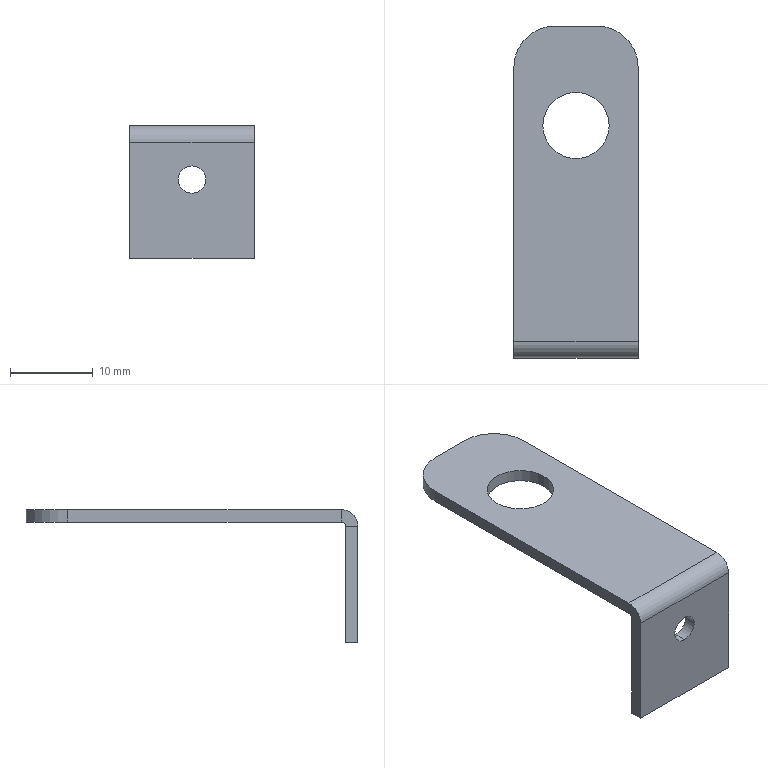Part | SolidWorks | features EdgeFlange 2, Fillet 2, FlatPattern 1, HoleWzd 1, ICE 1, SMBaseFlange 1, SheetMetal 1 | 1 solid | 20 faces | box 15 x 40 x 16 mm | volume 1110 mm3 | plane 12 | cylinder 8 | commonest cylinder face diameters 3.3 x2 8 x2 10 x2 1 x1 4 x1
STEP:
#1=CARTESIAN_POINT('',(4.,8.,0.));
#2=VERTEX_POINT('',#1);
#3=CARTESIAN_POINT('',(-4.,8.,0.));
#4=VERTEX_POINT('',#3);
#5=CARTESIAN_POINT('',(0.,8.,0.));
#6=DIRECTION('',(0.,0.,-1.));
#7=DIRECTION('',(-1.,0.,0.));
#8=AXIS2_PLACEMENT_3D('',#5,#6,#7);
#9=CIRCLE('',#8,4.);
#10=EDGE_CURVE('',#2,#4,#9,.T.);
#11=ORIENTED_EDGE('',*,*,#10,.F.);
#12=CARTESIAN_POINT('',(4.,8.,-1.5));
#13=VERTEX_POINT('',#12);
#14=CARTESIAN_POINT('',(4.,8.,0.));
#15=DIRECTION('',(0.,0.,-1.));
#16=VECTOR('',#15,1000.);
#17=LINE('',#14,#16);
#18=EDGE_CURVE('',#2,#13,#17,.T.);
#19=ORIENTED_EDGE('',*,*,#18,.T.);
#20=CARTESIAN_POINT('',(-4.,8.,-1.5));
#21=VERTEX_POINT('',#20);
#22=CARTESIAN_POINT('',(0.,8.,-1.5));
#23=DIRECTION('',(0.,0.,-1.));
#24=DIRECTION('',(-1.,0.,0.));
#25=AXIS2_PLACEMENT_3D('',#22,#23,#24);
#26=CIRCLE('',#25,4.);
#27=EDGE_CURVE('',#13,#21,#26,.T.);
#28=ORIENTED_EDGE('',*,*,#27,.T.);
#29=CARTESIAN_POINT('',(-4.,8.,0.));
#30=DIRECTION('',(0.,0.,-1.));
#31=VECTOR('',#30,1000.);
#32=LINE('',#29,#31);
#33=EDGE_CURVE('',#4,#21,#32,.T.);
#34=ORIENTED_EDGE('',*,*,#33,.F.);
#35=EDGE_LOOP('',(#11,#19,#28,#34));
#36=FACE_OUTER_BOUND('',#35,.T.);
#37=CARTESIAN_POINT('',(0.,8.,0.));
#38=DIRECTION('',(0.,0.,-1.));
#39=DIRECTION('',(-1.,0.,0.));
#40=AXIS2_PLACEMENT_3D('',#37,#38,#39);
#41=CYLINDRICAL_SURFACE('',#40,4.);
#42=ADVANCED_FACE('',(#36),#41,.F.);
#43=CARTESIAN_POINT('',(0.,-18.5,-4.85));
#44=VERTEX_POINT('',#43);
#45=CARTESIAN_POINT('',(0.,-18.5,-8.15));
#46=VERTEX_POINT('',#45);
#47=CARTESIAN_POINT('',(0.,-18.5,-6.5));
#48=DIRECTION('',(0.,-1.,0.));
#49=DIRECTION('',(0.,0.,-1.));
#50=AXIS2_PLACEMENT_3D('',#47,#48,#49);
#51=CIRCLE('',#50,1.65);
#52=EDGE_CURVE('',#44,#46,#51,.T.);
#53=ORIENTED_EDGE('',*,*,#52,.F.);
#54=CARTESIAN_POINT('',(0.,-20.,-4.85));
#55=VERTEX_POINT('',#54);
#56=CARTESIAN_POINT('',(0.,-20.,-4.85));
#57=DIRECTION('',(0.,-1.,0.));
#58=VECTOR('',#57,1000.);
#59=LINE('',#56,#58);
#60=EDGE_CURVE('',#44,#55,#59,.T.);
#61=ORIENTED_EDGE('',*,*,#60,.T.);
#62=CARTESIAN_POINT('',(0.,-20.,-8.15));
#63=VERTEX_POINT('',#62);
#64=CARTESIAN_POINT('',(0.,-20.,-6.5));
#65=DIRECTION('',(0.,-1.,0.));
#66=DIRECTION('',(0.,0.,-1.));
#67=AXIS2_PLACEMENT_3D('',#64,#65,#66);
#68=CIRCLE('',#67,1.65);
#69=EDGE_CURVE('',#55,#63,#68,.T.);
#70=ORIENTED_EDGE('',*,*,#69,.T.);
#71=CARTESIAN_POINT('',(0.,-20.,-8.15));
#72=DIRECTION('',(0.,-1.,0.));
#73=VECTOR('',#72,1000.);
#74=LINE('',#71,#73);
#75=EDGE_CURVE('',#46,#63,#74,.T.);
#76=ORIENTED_EDGE('',*,*,#75,.F.);
#77=EDGE_LOOP('',(#53,#61,#70,#76));
#78=FACE_OUTER_BOUND('',#77,.T.);
#79=CARTESIAN_POINT('',(0.,-20.,-6.5));
#80=DIRECTION('',(0.,-1.,0.));
#81=DIRECTION('',(0.,0.,-1.));
#82=AXIS2_PLACEMENT_3D('',#79,#80,#81);
#83=CYLINDRICAL_SURFACE('',#82,1.65);
#84=ADVANCED_FACE('',(#78),#83,.F.);
#85=CARTESIAN_POINT('',(-7.5,15.,-1.5));
#86=VERTEX_POINT('',#85);
#87=CARTESIAN_POINT('',(-7.5,-18.,-1.5));
#88=VERTEX_POINT('',#87);
#89=CARTESIAN_POINT('',(-7.5,-20.,-1.5));
#90=DIRECTION('',(0.,-1.,0.));
#91=VECTOR('',#90,1000.);
#92=LINE('',#89,#91);
#93=EDGE_CURVE('',#86,#88,#92,.T.);
#94=ORIENTED_EDGE('',*,*,#93,.T.);
#95=CARTESIAN_POINT('',(-7.5,-18.,0.));
#96=VERTEX_POINT('',#95);
#97=CARTESIAN_POINT('',(-7.5,-18.,-1.5));
#98=DIRECTION('',(0.,0.,1.));
#99=VECTOR('',#98,1000.);
#100=LINE('',#97,#99);
#101=EDGE_CURVE('',#88,#96,#100,.T.);
#102=ORIENTED_EDGE('',*,*,#101,.T.);
#103=CARTESIAN_POINT('',(-7.5,15.,0.));
#104=VERTEX_POINT('',#103);
#105=CARTESIAN_POINT('',(-7.5,-20.,0.));
#106=DIRECTION('',(0.,-1.,0.));
#107=VECTOR('',#106,1000.);
#108=LINE('',#105,#107);
#109=EDGE_CURVE('',#104,#96,#108,.T.);
#110=ORIENTED_EDGE('',*,*,#109,.F.);
#111=CARTESIAN_POINT('',(-7.5,15.,-1.5));
#112=DIRECTION('',(0.,0.,-1.));
#113=VECTOR('',#112,1000.);
#114=LINE('',#111,#113);
#115=EDGE_CURVE('',#104,#86,#114,.T.);
#116=ORIENTED_EDGE('',*,*,#115,.T.);
#117=EDGE_LOOP('',(#94,#102,#110,#116));
#118=FACE_OUTER_BOUND('',#117,.T.);
#119=CARTESIAN_POINT('',(-7.5,-20.,-1.5));
#120=DIRECTION('',(-1.,0.,0.));
#121=DIRECTION('',(0.,0.,1.));
#122=AXIS2_PLACEMENT_3D('',#119,#120,#121);
#123=PLANE('',#122);
#124=ADVANCED_FACE('',(#118),#123,.T.);
#125=CARTESIAN_POINT('',(0.,8.,-1.5));
#126=DIRECTION('',(0.,0.,-1.));
#127=DIRECTION('',(-1.,0.,0.));
#128=AXIS2_PLACEMENT_3D('',#125,#126,#127);
#129=CIRCLE('',#128,4.);
#130=EDGE_CURVE('',#21,#13,#129,.T.);
#131=ORIENTED_EDGE('',*,*,#130,.F.);
#132=ORIENTED_EDGE('',*,*,#27,.F.);
#133=EDGE_LOOP('',(#131,#132));
#134=FACE_BOUND('',#133,.T.);
#135=CARTESIAN_POINT('',(7.5,-18.,-1.5));
#136=VERTEX_POINT('',#135);
#137=CARTESIAN_POINT('',(-7.5,-18.,-1.5));
#138=DIRECTION('',(1.,0.,0.));
#139=VECTOR('',#138,1000.);
#140=LINE('',#137,#139);
#141=EDGE_CURVE('',#88,#136,#140,.T.);
#142=ORIENTED_EDGE('',*,*,#141,.F.);
#143=ORIENTED_EDGE('',*,*,#93,.F.);
#144=CARTESIAN_POINT('',(-2.5,20.,-1.5));
#145=VERTEX_POINT('',#144);
#146=CARTESIAN_POINT('',(-2.5,15.,-1.5));
#147=DIRECTION('',(0.,0.,-1.));
#148=DIRECTION('',(1.,0.,0.));
#149=AXIS2_PLACEMENT_3D('',#146,#147,#148);
#150=CIRCLE('',#149,5.);
#151=EDGE_CURVE('',#86,#145,#150,.T.);
#152=ORIENTED_EDGE('',*,*,#151,.T.);
#153=CARTESIAN_POINT('',(2.5,20.,-1.5));
#154=VERTEX_POINT('',#153);
#155=CARTESIAN_POINT('',(7.5,20.,-1.5));
#156=DIRECTION('',(-1.,0.,0.));
#157=VECTOR('',#156,1000.);
#158=LINE('',#155,#157);
#159=EDGE_CURVE('',#154,#145,#158,.T.);
#160=ORIENTED_EDGE('',*,*,#159,.F.);
#161=CARTESIAN_POINT('',(7.5,15.,-1.5));
#162=VERTEX_POINT('',#161);
#163=CARTESIAN_POINT('',(2.5,15.,-1.5));
#164=DIRECTION('',(0.,0.,-1.));
#165=DIRECTION('',(1.,0.,0.));
#166=AXIS2_PLACEMENT_3D('',#163,#164,#165);
#167=CIRCLE('',#166,5.);
#168=EDGE_CURVE('',#154,#162,#167,.T.);
#169=ORIENTED_EDGE('',*,*,#168,.T.);
#170=CARTESIAN_POINT('',(7.5,-20.,-1.5));
#171=DIRECTION('',(0.,1.,0.));
#172=VECTOR('',#171,1000.);
#173=LINE('',#170,#172);
#174=EDGE_CURVE('',#136,#162,#173,.T.);
#175=ORIENTED_EDGE('',*,*,#174,.F.);
#176=EDGE_LOOP('',(#142,#143,#152,#160,#169,#175));
#177=FACE_OUTER_BOUND('',#176,.T.);
#178=CARTESIAN_POINT('',(0.,0.,-1.5));
#179=DIRECTION('',(0.,0.,1.));
#180=DIRECTION('',(1.,0.,0.));
#181=AXIS2_PLACEMENT_3D('',#178,#179,#180);
#182=PLANE('',#181);
#183=ADVANCED_FACE('',(#134,#177),#182,.F.);
#184=CARTESIAN_POINT('',(0.,8.,0.));
#185=DIRECTION('',(0.,0.,-1.));
#186=DIRECTION('',(-1.,0.,0.));
#187=AXIS2_PLACEMENT_3D('',#184,#185,#186);
#188=CIRCLE('',#187,4.);
#189=EDGE_CURVE('',#4,#2,#188,.T.);
#190=ORIENTED_EDGE('',*,*,#189,.T.);
#191=ORIENTED_EDGE('',*,*,#10,.T.);
#192=EDGE_LOOP('',(#190,#191));
#193=FACE_BOUND('',#192,.T.);
#194=ORIENTED_EDGE('',*,*,#109,.T.);
#195=CARTESIAN_POINT('',(7.5,-18.,0.));
#196=VERTEX_POINT('',#195);
#197=CARTESIAN_POINT('',(-7.5,-18.,0.));
#198=DIRECTION('',(1.,0.,0.));
#199=VECTOR('',#198,1000.);
#200=LINE('',#197,#199);
#201=EDGE_CURVE('',#96,#196,#200,.T.);
#202=ORIENTED_EDGE('',*,*,#201,.T.);
#203=CARTESIAN_POINT('',(7.5,15.,0.));
#204=VERTEX_POINT('',#203);
#205=CARTESIAN_POINT('',(7.5,-20.,0.));
#206=DIRECTION('',(0.,1.,0.));
#207=VECTOR('',#206,1000.);
#208=LINE('',#205,#207);
#209=EDGE_CURVE('',#196,#204,#208,.T.);
#210=ORIENTED_EDGE('',*,*,#209,.T.);
#211=CARTESIAN_POINT('',(2.5,20.,0.));
#212=VERTEX_POINT('',#211);
#213=CARTESIAN_POINT('',(2.5,15.,0.));
#214=DIRECTION('',(0.,0.,1.));
#215=DIRECTION('',(1.,0.,0.));
#216=AXIS2_PLACEMENT_3D('',#213,#214,#215);
#217=CIRCLE('',#216,5.);
#218=EDGE_CURVE('',#204,#212,#217,.T.);
#219=ORIENTED_EDGE('',*,*,#218,.T.);
#220=CARTESIAN_POINT('',(-2.5,20.,0.));
#221=VERTEX_POINT('',#220);
#222=CARTESIAN_POINT('',(7.5,20.,0.));
#223=DIRECTION('',(-1.,0.,0.));
#224=VECTOR('',#223,1000.);
#225=LINE('',#222,#224);
#226=EDGE_CURVE('',#212,#221,#225,.T.);
#227=ORIENTED_EDGE('',*,*,#226,.T.);
#228=CARTESIAN_POINT('',(-2.5,15.,0.));
#229=DIRECTION('',(0.,0.,1.));
#230=DIRECTION('',(1.,0.,0.));
#231=AXIS2_PLACEMENT_3D('',#228,#229,#230);
#232=CIRCLE('',#231,5.);
#233=EDGE_CURVE('',#221,#104,#232,.T.);
#234=ORIENTED_EDGE('',*,*,#233,.T.);
#235=EDGE_LOOP('',(#194,#202,#210,#219,#227,#234));
#236=FACE_OUTER_BOUND('',#235,.T.);
#237=CARTESIAN_POINT('',(0.,0.,0.));
#238=DIRECTION('',(0.,0.,1.));
#239=DIRECTION('',(1.,0.,0.));
#240=AXIS2_PLACEMENT_3D('',#237,#238,#239);
#241=PLANE('',#240);
#242=ADVANCED_FACE('',(#193,#236),#241,.T.);
#243=ORIENTED_EDGE('',*,*,#226,.F.);
#244=CARTESIAN_POINT('',(2.5,20.,-1.5));
#245=DIRECTION('',(0.,0.,-1.));
#246=VECTOR('',#245,1000.);
#247=LINE('',#244,#246);
#248=EDGE_CURVE('',#212,#154,#247,.T.);
#249=ORIENTED_EDGE('',*,*,#248,.T.);
#250=ORIENTED_EDGE('',*,*,#159,.T.);
#251=CARTESIAN_POINT('',(-2.5,20.,-1.5));
#252=DIRECTION('',(0.,0.,1.));
#253=VECTOR('',#252,1000.);
#254=LINE('',#251,#253);
#255=EDGE_CURVE('',#145,#221,#254,.T.);
#256=ORIENTED_EDGE('',*,*,#255,.T.);
#257=EDGE_LOOP('',(#243,#249,#250,#256));
#258=FACE_OUTER_BOUND('',#257,.T.);
#259=CARTESIAN_POINT('',(7.5,20.,-1.5));
#260=DIRECTION('',(0.,1.,0.));
#261=DIRECTION('',(0.,0.,1.));
#262=AXIS2_PLACEMENT_3D('',#259,#260,#261);
#263=PLANE('',#262);
#264=ADVANCED_FACE('',(#258),#263,.T.);
#265=CARTESIAN_POINT('',(7.5,-18.,-1.5));
#266=DIRECTION('',(0.,0.,1.));
#267=VECTOR('',#266,1000.);
#268=LINE('',#265,#267);
#269=EDGE_CURVE('',#136,#196,#268,.T.);
#270=ORIENTED_EDGE('',*,*,#269,.F.);
#271=ORIENTED_EDGE('',*,*,#174,.T.);
#272=CARTESIAN_POINT('',(7.5,15.,-1.5));
#273=DIRECTION('',(0.,0.,1.));
#274=VECTOR('',#273,1000.);
#275=LINE('',#272,#274);
#276=EDGE_CURVE('',#162,#204,#275,.T.);
#277=ORIENTED_EDGE('',*,*,#276,.T.);
#278=ORIENTED_EDGE('',*,*,#209,.F.);
#279=EDGE_LOOP('',(#270,#271,#277,#278));
#280=FACE_OUTER_BOUND('',#279,.T.);
#281=CARTESIAN_POINT('',(7.5,-20.,-1.5));
#282=DIRECTION('',(1.,0.,0.));
#283=DIRECTION('',(0.,0.,-1.));
#284=AXIS2_PLACEMENT_3D('',#281,#282,#283);
#285=PLANE('',#284);
#286=ADVANCED_FACE('',(#280),#285,.T.);
#287=ORIENTED_EDGE('',*,*,#168,.F.);
#288=ORIENTED_EDGE('',*,*,#248,.F.);
#289=ORIENTED_EDGE('',*,*,#218,.F.);
#290=ORIENTED_EDGE('',*,*,#276,.F.);
#291=EDGE_LOOP('',(#287,#288,#289,#290));
#292=FACE_OUTER_BOUND('',#291,.T.);
#293=CARTESIAN_POINT('',(2.5,15.,-1.5));
#294=DIRECTION('',(0.,0.,1.));
#295=DIRECTION('',(1.,0.,0.));
#296=AXIS2_PLACEMENT_3D('',#293,#294,#295);
#297=CYLINDRICAL_SURFACE('',#296,5.);
#298=ADVANCED_FACE('',(#292),#297,.T.);
#299=ORIENTED_EDGE('',*,*,#151,.F.);
#300=ORIENTED_EDGE('',*,*,#115,.F.);
#301=ORIENTED_EDGE('',*,*,#233,.F.);
#302=ORIENTED_EDGE('',*,*,#255,.F.);
#303=EDGE_LOOP('',(#299,#300,#301,#302));
#304=FACE_OUTER_BOUND('',#303,.T.);
#305=CARTESIAN_POINT('',(-2.5,15.,-1.5));
#306=DIRECTION('',(0.,0.,1.));
#307=DIRECTION('',(1.,0.,0.));
#308=AXIS2_PLACEMENT_3D('',#305,#306,#307);
#309=CYLINDRICAL_SURFACE('',#308,5.);
#310=ADVANCED_FACE('',(#304),#309,.T.);
#311=CARTESIAN_POINT('',(7.5,-18.5,-2.));
#312=VERTEX_POINT('',#311);
#313=CARTESIAN_POINT('',(7.5,-20.,-2.));
#314=VERTEX_POINT('',#313);
#315=CARTESIAN_POINT('',(7.5,-20.,-2.));
#316=DIRECTION('',(0.,-1.,0.));
#317=VECTOR('',#316,1000.);
#318=LINE('',#315,#317);
#319=EDGE_CURVE('',#312,#314,#318,.T.);
#320=ORIENTED_EDGE('',*,*,#319,.F.);
#321=CARTESIAN_POINT('',(7.5,-18.,-2.));
#322=DIRECTION('',(1.,0.,0.));
#323=DIRECTION('',(0.,0.,1.));
#324=AXIS2_PLACEMENT_3D('',#321,#322,#323);
#325=CIRCLE('',#324,0.5);
#326=EDGE_CURVE('',#136,#312,#325,.T.);
#327=ORIENTED_EDGE('',*,*,#326,.F.);
#328=ORIENTED_EDGE('',*,*,#269,.T.);
#329=CARTESIAN_POINT('',(7.5,-18.,-2.));
#330=DIRECTION('',(1.,0.,0.));
#331=DIRECTION('',(0.,0.,1.));
#332=AXIS2_PLACEMENT_3D('',#329,#330,#331);
#333=CIRCLE('',#332,2.);
#334=EDGE_CURVE('',#196,#314,#333,.T.);
#335=ORIENTED_EDGE('',*,*,#334,.T.);
#336=EDGE_LOOP('',(#320,#327,#328,#335));
#337=FACE_OUTER_BOUND('',#336,.T.);
#338=CARTESIAN_POINT('',(7.5,-18.,-2.));
#339=DIRECTION('',(1.,0.,0.));
#340=DIRECTION('',(0.,0.,-1.));
#341=AXIS2_PLACEMENT_3D('',#338,#339,#340);
#342=PLANE('',#341);
#343=ADVANCED_FACE('',(#337),#342,.T.);
#344=CARTESIAN_POINT('',(-7.5,-18.5,-2.));
#345=VERTEX_POINT('',#344);
#346=CARTESIAN_POINT('',(-7.5,-18.,-2.));
#347=DIRECTION('',(-1.,0.,0.));
#348=DIRECTION('',(0.,0.,1.));
#349=AXIS2_PLACEMENT_3D('',#346,#347,#348);
#350=CIRCLE('',#349,0.5);
#351=EDGE_CURVE('',#345,#88,#350,.T.);
#352=ORIENTED_EDGE('',*,*,#351,.F.);
#353=CARTESIAN_POINT('',(-7.5,-20.,-2.));
#354=VERTEX_POINT('',#353);
#355=CARTESIAN_POINT('',(-7.5,-18.5,-2.));
#356=DIRECTION('',(0.,-1.,0.));
#357=VECTOR('',#356,1000.);
#358=LINE('',#355,#357);
#359=EDGE_CURVE('',#345,#354,#358,.T.);
#360=ORIENTED_EDGE('',*,*,#359,.T.);
#361=CARTESIAN_POINT('',(-7.5,-18.,-2.));
#362=DIRECTION('',(-1.,0.,0.));
#363=DIRECTION('',(0.,0.,1.));
#364=AXIS2_PLACEMENT_3D('',#361,#362,#363);
#365=CIRCLE('',#364,2.);
#366=EDGE_CURVE('',#354,#96,#365,.T.);
#367=ORIENTED_EDGE('',*,*,#366,.T.);
#368=ORIENTED_EDGE('',*,*,#101,.F.);
#369=EDGE_LOOP('',(#352,#360,#367,#368));
#370=FACE_OUTER_BOUND('',#369,.T.);
#371=CARTESIAN_POINT('',(-7.5,-18.,-2.));
#372=DIRECTION('',(1.,0.,0.));
#373=DIRECTION('',(0.,0.,-1.));
#374=AXIS2_PLACEMENT_3D('',#371,#372,#373);
#375=PLANE('',#374);
#376=ADVANCED_FACE('',(#370),#375,.F.);
#377=ORIENTED_EDGE('',*,*,#201,.F.);
#378=ORIENTED_EDGE('',*,*,#366,.F.);
#379=CARTESIAN_POINT('',(0.,-20.,-2.));
#380=DIRECTION('',(-1.,0.,0.));
#381=VECTOR('',#380,1000.);
#382=LINE('',#379,#381);
#383=EDGE_CURVE('',#314,#354,#382,.T.);
#384=ORIENTED_EDGE('',*,*,#383,.F.);
#385=ORIENTED_EDGE('',*,*,#334,.F.);
#386=EDGE_LOOP('',(#377,#378,#384,#385));
#387=FACE_OUTER_BOUND('',#386,.T.);
#388=CARTESIAN_POINT('',(-7.5,-18.,-2.));
#389=DIRECTION('',(-1.,0.,0.));
#390=DIRECTION('',(0.,-1.,0.));
#391=AXIS2_PLACEMENT_3D('',#388,#389,#390);
#392=CYLINDRICAL_SURFACE('',#391,2.);
#393=ADVANCED_FACE('',(#387),#392,.T.);
#394=ORIENTED_EDGE('',*,*,#141,.T.);
#395=ORIENTED_EDGE('',*,*,#326,.T.);
#396=CARTESIAN_POINT('',(7.5,-18.5,-2.));
#397=DIRECTION('',(-1.,0.,0.));
#398=VECTOR('',#397,1000.);
#399=LINE('',#396,#398);
#400=EDGE_CURVE('',#312,#345,#399,.T.);
#401=ORIENTED_EDGE('',*,*,#400,.T.);
#402=ORIENTED_EDGE('',*,*,#351,.T.);
#403=EDGE_LOOP('',(#394,#395,#401,#402));
#404=FACE_OUTER_BOUND('',#403,.T.);
#405=CARTESIAN_POINT('',(-7.5,-18.,-2.));
#406=DIRECTION('',(-1.,0.,0.));
#407=DIRECTION('',(0.,-1.,0.));
#408=AXIS2_PLACEMENT_3D('',#405,#406,#407);
#409=CYLINDRICAL_SURFACE('',#408,0.5);
#410=ADVANCED_FACE('',(#404),#409,.F.);
#411=CARTESIAN_POINT('',(-7.5,-20.,-16.));
#412=VERTEX_POINT('',#411);
#413=CARTESIAN_POINT('',(-7.5,-20.,-1.5));
#414=DIRECTION('',(0.,0.,1.));
#415=VECTOR('',#414,1000.);
#416=LINE('',#413,#415);
#417=EDGE_CURVE('',#412,#354,#416,.T.);
#418=ORIENTED_EDGE('',*,*,#417,.T.);
#419=ORIENTED_EDGE('',*,*,#359,.F.);
#420=CARTESIAN_POINT('',(-7.5,-18.5,-16.));
#421=VERTEX_POINT('',#420);
#422=CARTESIAN_POINT('',(-7.5,-18.5,0.));
#423=DIRECTION('',(0.,0.,1.));
#424=VECTOR('',#423,1000.);
#425=LINE('',#422,#424);
#426=EDGE_CURVE('',#421,#345,#425,.T.);
#427=ORIENTED_EDGE('',*,*,#426,.F.);
#428=CARTESIAN_POINT('',(-7.5,-20.,-16.));
#429=DIRECTION('',(0.,1.,0.));
#430=VECTOR('',#429,1000.);
#431=LINE('',#428,#430);
#432=EDGE_CURVE('',#412,#421,#431,.T.);
#433=ORIENTED_EDGE('',*,*,#432,.F.);
#434=EDGE_LOOP('',(#418,#419,#427,#433));
#435=FACE_OUTER_BOUND('',#434,.T.);
#436=CARTESIAN_POINT('',(-7.5,-20.,-1.5));
#437=DIRECTION('',(-1.,0.,0.));
#438=DIRECTION('',(0.,0.,1.));
#439=AXIS2_PLACEMENT_3D('',#436,#437,#438);
#440=PLANE('',#439);
#441=ADVANCED_FACE('',(#435),#440,.T.);
#442=CARTESIAN_POINT('',(7.5,-18.5,-16.));
#443=VERTEX_POINT('',#442);
#444=CARTESIAN_POINT('',(7.5,-18.5,0.));
#445=DIRECTION('',(0.,0.,-1.));
#446=VECTOR('',#445,1000.);
#447=LINE('',#444,#446);
#448=EDGE_CURVE('',#312,#443,#447,.T.);
#449=ORIENTED_EDGE('',*,*,#448,.F.);
#450=ORIENTED_EDGE('',*,*,#319,.T.);
#451=CARTESIAN_POINT('',(7.5,-20.,-16.));
#452=VERTEX_POINT('',#451);
#453=CARTESIAN_POINT('',(7.5,-20.,-16.));
#454=DIRECTION('',(0.,0.,-1.));
#455=VECTOR('',#454,1000.);
#456=LINE('',#453,#455);
#457=EDGE_CURVE('',#314,#452,#456,.T.);
#458=ORIENTED_EDGE('',*,*,#457,.T.);
#459=CARTESIAN_POINT('',(7.5,-20.,-16.));
#460=DIRECTION('',(0.,1.,0.));
#461=VECTOR('',#460,1000.);
#462=LINE('',#459,#461);
#463=EDGE_CURVE('',#452,#443,#462,.T.);
#464=ORIENTED_EDGE('',*,*,#463,.T.);
#465=EDGE_LOOP('',(#449,#450,#458,#464));
#466=FACE_OUTER_BOUND('',#465,.T.);
#467=CARTESIAN_POINT('',(7.5,-20.,-16.));
#468=DIRECTION('',(1.,0.,0.));
#469=DIRECTION('',(0.,0.,-1.));
#470=AXIS2_PLACEMENT_3D('',#467,#468,#469);
#471=PLANE('',#470);
#472=ADVANCED_FACE('',(#466),#471,.T.);
#473=CARTESIAN_POINT('',(0.,-20.,-6.5));
#474=DIRECTION('',(0.,-1.,0.));
#475=DIRECTION('',(0.,0.,-1.));
#476=AXIS2_PLACEMENT_3D('',#473,#474,#475);
#477=CIRCLE('',#476,1.65);
#478=EDGE_CURVE('',#63,#55,#477,.T.);
#479=ORIENTED_EDGE('',*,*,#478,.F.);
#480=ORIENTED_EDGE('',*,*,#69,.F.);
#481=EDGE_LOOP('',(#479,#480));
#482=FACE_BOUND('',#481,.T.);
#483=ORIENTED_EDGE('',*,*,#457,.F.);
#484=ORIENTED_EDGE('',*,*,#383,.T.);
#485=ORIENTED_EDGE('',*,*,#417,.F.);
#486=CARTESIAN_POINT('',(-7.5,-20.,-16.));
#487=DIRECTION('',(-1.,0.,0.));
#488=VECTOR('',#487,1000.);
#489=LINE('',#486,#488);
#490=EDGE_CURVE('',#452,#412,#489,.T.);
#491=ORIENTED_EDGE('',*,*,#490,.F.);
#492=EDGE_LOOP('',(#483,#484,#485,#491));
#493=FACE_OUTER_BOUND('',#492,.T.);
#494=CARTESIAN_POINT('',(0.,-20.,0.));
#495=DIRECTION('',(0.,-1.,0.));
#496=DIRECTION('',(0.,0.,-1.));
#497=AXIS2_PLACEMENT_3D('',#494,#495,#496);
#498=PLANE('',#497);
#499=ADVANCED_FACE('',(#482,#493),#498,.T.);
#500=CARTESIAN_POINT('',(0.,-18.5,-6.5));
#501=DIRECTION('',(0.,-1.,0.));
#502=DIRECTION('',(0.,0.,-1.));
#503=AXIS2_PLACEMENT_3D('',#500,#501,#502);
#504=CIRCLE('',#503,1.65);
#505=EDGE_CURVE('',#46,#44,#504,.T.);
#506=ORIENTED_EDGE('',*,*,#505,.T.);
#507=ORIENTED_EDGE('',*,*,#52,.T.);
#508=EDGE_LOOP('',(#506,#507));
#509=FACE_BOUND('',#508,.T.);
#510=ORIENTED_EDGE('',*,*,#400,.F.);
#511=ORIENTED_EDGE('',*,*,#448,.T.);
#512=CARTESIAN_POINT('',(0.,-18.5,-16.));
#513=DIRECTION('',(-1.,0.,0.));
#514=VECTOR('',#513,1000.);
#515=LINE('',#512,#514);
#516=EDGE_CURVE('',#443,#421,#515,.T.);
#517=ORIENTED_EDGE('',*,*,#516,.T.);
#518=ORIENTED_EDGE('',*,*,#426,.T.);
#519=EDGE_LOOP('',(#510,#511,#517,#518));
#520=FACE_OUTER_BOUND('',#519,.T.);
#521=CARTESIAN_POINT('',(0.,-18.5,0.));
#522=DIRECTION('',(0.,-1.,0.));
#523=DIRECTION('',(0.,0.,-1.));
#524=AXIS2_PLACEMENT_3D('',#521,#522,#523);
#525=PLANE('',#524);
#526=ADVANCED_FACE('',(#509,#520),#525,.F.);
#527=ORIENTED_EDGE('',*,*,#516,.F.);
#528=ORIENTED_EDGE('',*,*,#463,.F.);
#529=ORIENTED_EDGE('',*,*,#490,.T.);
#530=ORIENTED_EDGE('',*,*,#432,.T.);
#531=EDGE_LOOP('',(#527,#528,#529,#530));
#532=FACE_OUTER_BOUND('',#531,.T.);
#533=CARTESIAN_POINT('',(-7.5,-20.,-16.));
#534=DIRECTION('',(0.,0.,-1.));
#535=DIRECTION('',(0.,1.,0.));
#536=AXIS2_PLACEMENT_3D('',#533,#534,#535);
#537=PLANE('',#536);
#538=ADVANCED_FACE('',(#532),#537,.T.);
#539=ORIENTED_EDGE('',*,*,#60,.F.);
#540=ORIENTED_EDGE('',*,*,#505,.F.);
#541=ORIENTED_EDGE('',*,*,#75,.T.);
#542=ORIENTED_EDGE('',*,*,#478,.T.);
#543=EDGE_LOOP('',(#539,#540,#541,#542));
#544=FACE_OUTER_BOUND('',#543,.T.);
#545=CARTESIAN_POINT('',(0.,-20.,-6.5));
#546=DIRECTION('',(0.,-1.,0.));
#547=DIRECTION('',(0.,0.,-1.));
#548=AXIS2_PLACEMENT_3D('',#545,#546,#547);
#549=CYLINDRICAL_SURFACE('',#548,1.65);
#550=ADVANCED_FACE('',(#544),#549,.F.);
#551=ORIENTED_EDGE('',*,*,#18,.F.);
#552=ORIENTED_EDGE('',*,*,#189,.F.);
#553=ORIENTED_EDGE('',*,*,#33,.T.);
#554=ORIENTED_EDGE('',*,*,#130,.T.);
#555=EDGE_LOOP('',(#551,#552,#553,#554));
#556=FACE_OUTER_BOUND('',#555,.T.);
#557=CARTESIAN_POINT('',(0.,8.,0.));
#558=DIRECTION('',(0.,0.,-1.));
#559=DIRECTION('',(-1.,0.,0.));
#560=AXIS2_PLACEMENT_3D('',#557,#558,#559);
#561=CYLINDRICAL_SURFACE('',#560,4.);
#562=ADVANCED_FACE('',(#556),#561,.F.);
#563=CLOSED_SHELL('',(#42,#84,#124,#183,#242,#264,#286,#298,#310,#343,#376,#393,#410,#441,#472,#499,#526,#538,#550,#562));
#564=MANIFOLD_SOLID_BREP('',#563);
#565=CARTESIAN_POINT('',(0.,0.,0.));
#566=DIRECTION('',(0.,0.,1.));
#567=DIRECTION('',(1.,0.,0.));
#568=AXIS2_PLACEMENT_3D('',#565,#566,#567);
#569=(LENGTH_UNIT()NAMED_UNIT(*)SI_UNIT(.MILLI.,.METRE.));
#570=UNCERTAINTY_MEASURE_WITH_UNIT(LENGTH_MEASURE(0.00001),#569,'','');
#571=(NAMED_UNIT(*)PLANE_ANGLE_UNIT()SI_UNIT($,.RADIAN.));
#572=(NAMED_UNIT(*)SI_UNIT($,.STERADIAN.)SOLID_ANGLE_UNIT());
#573=(GEOMETRIC_REPRESENTATION_CONTEXT(3)GLOBAL_UNCERTAINTY_ASSIGNED_CONTEXT((#570))GLOBAL_UNIT_ASSIGNED_CONTEXT((#569,#571,#572))REPRESENTATION_CONTEXT('',''));
#574=ADVANCED_BREP_SHAPE_REPRESENTATION('',(#564,#568),#573);